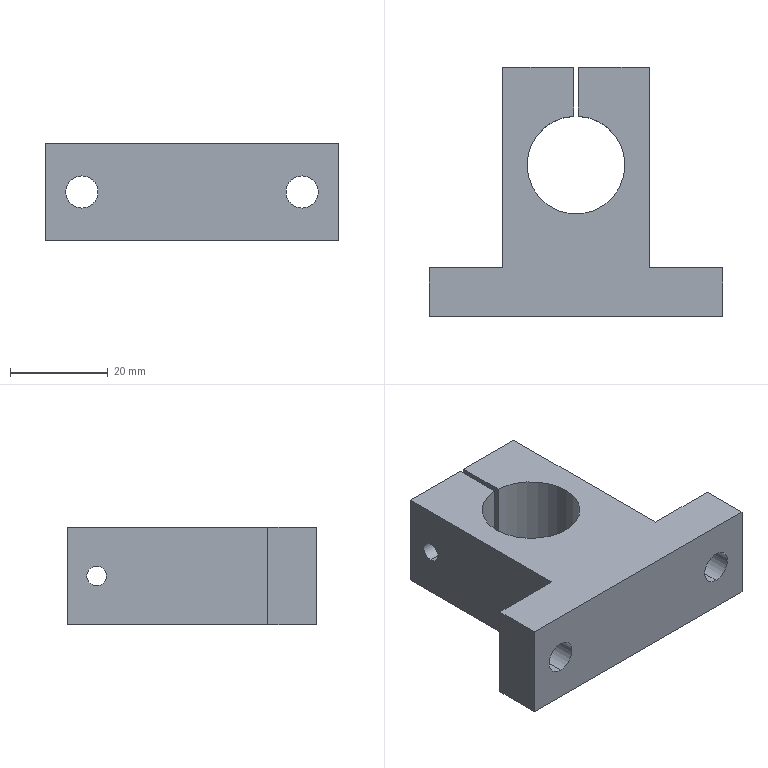Part | SolidWorks | features HoleWzd 3, Extrusion 1, RefAxis 1 | 1 solid | 27 faces | box 60 x 51 x 20 mm | volume 28604 mm3 | plane 14 | cylinder 13 | commonest cylinder face diameters 6.6 x4 20 x3 4 x2 5.5 x2 10 x2
STEP:
#1=CARTESIAN_POINT('',(-15.,45.,2.));
#2=VERTEX_POINT('',#1);
#3=CARTESIAN_POINT('',(-15.,45.,-2.));
#4=VERTEX_POINT('',#3);
#5=CARTESIAN_POINT('',(-15.,45.,0.));
#6=DIRECTION('',(1.,0.,0.));
#7=DIRECTION('',(0.,1.,0.));
#8=AXIS2_PLACEMENT_3D('',#5,#6,#7);
#9=CIRCLE('',#8,2.);
#10=EDGE_CURVE('',#2,#4,#9,.T.);
#11=ORIENTED_EDGE('',*,*,#10,.F.);
#12=CARTESIAN_POINT('',(-0.5,45.,2.));
#13=VERTEX_POINT('',#12);
#14=CARTESIAN_POINT('',(-0.5,45.,2.));
#15=DIRECTION('',(1.,0.,0.));
#16=VECTOR('',#15,1000.);
#17=LINE('',#14,#16);
#18=EDGE_CURVE('',#2,#13,#17,.T.);
#19=ORIENTED_EDGE('',*,*,#18,.T.);
#20=CARTESIAN_POINT('',(-0.5,45.,-2.));
#21=VERTEX_POINT('',#20);
#22=CARTESIAN_POINT('',(-0.5,45.,0.));
#23=DIRECTION('',(1.,0.,0.));
#24=DIRECTION('',(0.,0.,-1.));
#25=AXIS2_PLACEMENT_3D('',#22,#23,#24);
#26=CIRCLE('',#25,2.);
#27=EDGE_CURVE('',#13,#21,#26,.T.);
#28=ORIENTED_EDGE('',*,*,#27,.T.);
#29=CARTESIAN_POINT('',(-0.5,45.,-2.));
#30=DIRECTION('',(1.,0.,0.));
#31=VECTOR('',#30,1000.);
#32=LINE('',#29,#31);
#33=EDGE_CURVE('',#4,#21,#32,.T.);
#34=ORIENTED_EDGE('',*,*,#33,.F.);
#35=EDGE_LOOP('',(#11,#19,#28,#34));
#36=FACE_OUTER_BOUND('',#35,.T.);
#37=CARTESIAN_POINT('',(-0.5,45.,0.));
#38=DIRECTION('',(1.,0.,0.));
#39=DIRECTION('',(0.,0.,-1.));
#40=AXIS2_PLACEMENT_3D('',#37,#38,#39);
#41=CYLINDRICAL_SURFACE('',#40,2.);
#42=ADVANCED_FACE('',(#36),#41,.F.);
#43=CARTESIAN_POINT('',(-22.5,0.,-3.3));
#44=VERTEX_POINT('',#43);
#45=CARTESIAN_POINT('',(-22.5,0.,3.3));
#46=VERTEX_POINT('',#45);
#47=CARTESIAN_POINT('',(-22.5,0.,0.));
#48=DIRECTION('',(0.,1.,0.));
#49=DIRECTION('',(0.,0.,1.));
#50=AXIS2_PLACEMENT_3D('',#47,#48,#49);
#51=CIRCLE('',#50,3.3);
#52=EDGE_CURVE('',#44,#46,#51,.T.);
#53=ORIENTED_EDGE('',*,*,#52,.F.);
#54=CARTESIAN_POINT('',(-22.5,10.,-3.3));
#55=VERTEX_POINT('',#54);
#56=CARTESIAN_POINT('',(-22.5,10.,-3.3));
#57=DIRECTION('',(0.,1.,0.));
#58=VECTOR('',#57,1000.);
#59=LINE('',#56,#58);
#60=EDGE_CURVE('',#44,#55,#59,.T.);
#61=ORIENTED_EDGE('',*,*,#60,.T.);
#62=CARTESIAN_POINT('',(-22.5,10.,3.3));
#63=VERTEX_POINT('',#62);
#64=CARTESIAN_POINT('',(-22.5,10.,0.));
#65=DIRECTION('',(0.,1.,0.));
#66=DIRECTION('',(0.,0.,1.));
#67=AXIS2_PLACEMENT_3D('',#64,#65,#66);
#68=CIRCLE('',#67,3.3);
#69=EDGE_CURVE('',#55,#63,#68,.T.);
#70=ORIENTED_EDGE('',*,*,#69,.T.);
#71=CARTESIAN_POINT('',(-22.5,10.,3.3));
#72=DIRECTION('',(0.,1.,0.));
#73=VECTOR('',#72,1000.);
#74=LINE('',#71,#73);
#75=EDGE_CURVE('',#46,#63,#74,.T.);
#76=ORIENTED_EDGE('',*,*,#75,.F.);
#77=EDGE_LOOP('',(#53,#61,#70,#76));
#78=FACE_OUTER_BOUND('',#77,.T.);
#79=CARTESIAN_POINT('',(-22.5,10.,0.));
#80=DIRECTION('',(0.,1.,0.));
#81=DIRECTION('',(0.,0.,1.));
#82=AXIS2_PLACEMENT_3D('',#79,#80,#81);
#83=CYLINDRICAL_SURFACE('',#82,3.3);
#84=ADVANCED_FACE('',(#78),#83,.F.);
#85=CARTESIAN_POINT('',(22.5,0.,-3.3));
#86=VERTEX_POINT('',#85);
#87=CARTESIAN_POINT('',(22.5,0.,3.3));
#88=VERTEX_POINT('',#87);
#89=CARTESIAN_POINT('',(22.5,0.,0.));
#90=DIRECTION('',(0.,1.,0.));
#91=DIRECTION('',(0.,0.,1.));
#92=AXIS2_PLACEMENT_3D('',#89,#90,#91);
#93=CIRCLE('',#92,3.3);
#94=EDGE_CURVE('',#86,#88,#93,.T.);
#95=ORIENTED_EDGE('',*,*,#94,.F.);
#96=CARTESIAN_POINT('',(22.5,10.,-3.3));
#97=VERTEX_POINT('',#96);
#98=CARTESIAN_POINT('',(22.5,10.,-3.3));
#99=DIRECTION('',(0.,1.,0.));
#100=VECTOR('',#99,1000.);
#101=LINE('',#98,#100);
#102=EDGE_CURVE('',#86,#97,#101,.T.);
#103=ORIENTED_EDGE('',*,*,#102,.T.);
#104=CARTESIAN_POINT('',(22.5,10.,3.3));
#105=VERTEX_POINT('',#104);
#106=CARTESIAN_POINT('',(22.5,10.,0.));
#107=DIRECTION('',(0.,1.,0.));
#108=DIRECTION('',(0.,0.,1.));
#109=AXIS2_PLACEMENT_3D('',#106,#107,#108);
#110=CIRCLE('',#109,3.3);
#111=EDGE_CURVE('',#97,#105,#110,.T.);
#112=ORIENTED_EDGE('',*,*,#111,.T.);
#113=CARTESIAN_POINT('',(22.5,10.,3.3));
#114=DIRECTION('',(0.,1.,0.));
#115=VECTOR('',#114,1000.);
#116=LINE('',#113,#115);
#117=EDGE_CURVE('',#88,#105,#116,.T.);
#118=ORIENTED_EDGE('',*,*,#117,.F.);
#119=EDGE_LOOP('',(#95,#103,#112,#118));
#120=FACE_OUTER_BOUND('',#119,.T.);
#121=CARTESIAN_POINT('',(22.5,10.,0.));
#122=DIRECTION('',(0.,1.,0.));
#123=DIRECTION('',(0.,0.,1.));
#124=AXIS2_PLACEMENT_3D('',#121,#122,#123);
#125=CYLINDRICAL_SURFACE('',#124,3.3);
#126=ADVANCED_FACE('',(#120),#125,.F.);
#127=CARTESIAN_POINT('',(9.5,45.,5.));
#128=VERTEX_POINT('',#127);
#129=CARTESIAN_POINT('',(9.5,45.,-5.));
#130=VERTEX_POINT('',#129);
#131=CARTESIAN_POINT('',(9.5,45.,0.));
#132=DIRECTION('',(1.,0.,0.));
#133=DIRECTION('',(0.,0.,-1.));
#134=AXIS2_PLACEMENT_3D('',#131,#132,#133);
#135=CIRCLE('',#134,5.);
#136=EDGE_CURVE('',#128,#130,#135,.T.);
#137=ORIENTED_EDGE('',*,*,#136,.F.);
#138=CARTESIAN_POINT('',(15.,45.,5.));
#139=VERTEX_POINT('',#138);
#140=CARTESIAN_POINT('',(15.,45.,5.));
#141=DIRECTION('',(1.,0.,0.));
#142=VECTOR('',#141,1000.);
#143=LINE('',#140,#142);
#144=EDGE_CURVE('',#128,#139,#143,.T.);
#145=ORIENTED_EDGE('',*,*,#144,.T.);
#146=CARTESIAN_POINT('',(15.,45.,-5.));
#147=VERTEX_POINT('',#146);
#148=CARTESIAN_POINT('',(15.,45.,0.));
#149=DIRECTION('',(1.,0.,0.));
#150=DIRECTION('',(0.,0.,-1.));
#151=AXIS2_PLACEMENT_3D('',#148,#149,#150);
#152=CIRCLE('',#151,5.);
#153=EDGE_CURVE('',#139,#147,#152,.T.);
#154=ORIENTED_EDGE('',*,*,#153,.T.);
#155=CARTESIAN_POINT('',(15.,45.,-5.));
#156=DIRECTION('',(1.,0.,0.));
#157=VECTOR('',#156,1000.);
#158=LINE('',#155,#157);
#159=EDGE_CURVE('',#130,#147,#158,.T.);
#160=ORIENTED_EDGE('',*,*,#159,.F.);
#161=EDGE_LOOP('',(#137,#145,#154,#160));
#162=FACE_OUTER_BOUND('',#161,.T.);
#163=CARTESIAN_POINT('',(15.,45.,0.));
#164=DIRECTION('',(1.,0.,0.));
#165=DIRECTION('',(0.,0.,-1.));
#166=AXIS2_PLACEMENT_3D('',#163,#164,#165);
#167=CYLINDRICAL_SURFACE('',#166,5.);
#168=ADVANCED_FACE('',(#162),#167,.F.);
#169=CARTESIAN_POINT('',(0.5,45.,2.75));
#170=VERTEX_POINT('',#169);
#171=CARTESIAN_POINT('',(0.5,45.,-2.75));
#172=VERTEX_POINT('',#171);
#173=CARTESIAN_POINT('',(0.5,45.,0.));
#174=DIRECTION('',(1.,0.,0.));
#175=DIRECTION('',(0.,1.,0.));
#176=AXIS2_PLACEMENT_3D('',#173,#174,#175);
#177=CIRCLE('',#176,2.75);
#178=EDGE_CURVE('',#170,#172,#177,.T.);
#179=ORIENTED_EDGE('',*,*,#178,.F.);
#180=CARTESIAN_POINT('',(9.5,45.,2.75));
#181=VERTEX_POINT('',#180);
#182=CARTESIAN_POINT('',(15.,45.,2.75));
#183=DIRECTION('',(1.,0.,0.));
#184=VECTOR('',#183,1000.);
#185=LINE('',#182,#184);
#186=EDGE_CURVE('',#170,#181,#185,.T.);
#187=ORIENTED_EDGE('',*,*,#186,.T.);
#188=CARTESIAN_POINT('',(9.5,45.,-2.75));
#189=VERTEX_POINT('',#188);
#190=CARTESIAN_POINT('',(9.5,45.,0.));
#191=DIRECTION('',(1.,0.,0.));
#192=DIRECTION('',(0.,0.,-1.));
#193=AXIS2_PLACEMENT_3D('',#190,#191,#192);
#194=CIRCLE('',#193,2.75);
#195=EDGE_CURVE('',#181,#189,#194,.T.);
#196=ORIENTED_EDGE('',*,*,#195,.T.);
#197=CARTESIAN_POINT('',(15.,45.,-2.75));
#198=DIRECTION('',(1.,0.,0.));
#199=VECTOR('',#198,1000.);
#200=LINE('',#197,#199);
#201=EDGE_CURVE('',#172,#189,#200,.T.);
#202=ORIENTED_EDGE('',*,*,#201,.F.);
#203=EDGE_LOOP('',(#179,#187,#196,#202));
#204=FACE_OUTER_BOUND('',#203,.T.);
#205=CARTESIAN_POINT('',(15.,45.,0.));
#206=DIRECTION('',(1.,0.,0.));
#207=DIRECTION('',(0.,0.,-1.));
#208=AXIS2_PLACEMENT_3D('',#205,#206,#207);
#209=CYLINDRICAL_SURFACE('',#208,2.75);
#210=ADVANCED_FACE('',(#204),#209,.F.);
#211=CARTESIAN_POINT('',(10.,31.,10.));
#212=VERTEX_POINT('',#211);
#213=CARTESIAN_POINT('',(-10.,31.,10.));
#214=VERTEX_POINT('',#213);
#215=CARTESIAN_POINT('',(0.,31.,10.));
#216=DIRECTION('',(0.,0.,-1.));
#217=DIRECTION('',(1.,0.,0.));
#218=AXIS2_PLACEMENT_3D('',#215,#216,#217);
#219=CIRCLE('',#218,10.);
#220=EDGE_CURVE('',#212,#214,#219,.T.);
#221=ORIENTED_EDGE('',*,*,#220,.F.);
#222=CARTESIAN_POINT('',(10.,31.,-10.));
#223=VERTEX_POINT('',#222);
#224=CARTESIAN_POINT('',(10.,31.,10.));
#225=DIRECTION('',(0.,0.,-1.));
#226=VECTOR('',#225,1000.);
#227=LINE('',#224,#226);
#228=EDGE_CURVE('',#212,#223,#227,.T.);
#229=ORIENTED_EDGE('',*,*,#228,.T.);
#230=CARTESIAN_POINT('',(-10.,31.,-10.));
#231=VERTEX_POINT('',#230);
#232=CARTESIAN_POINT('',(0.,31.,-10.));
#233=DIRECTION('',(0.,0.,-1.));
#234=DIRECTION('',(1.,0.,0.));
#235=AXIS2_PLACEMENT_3D('',#232,#233,#234);
#236=CIRCLE('',#235,10.);
#237=EDGE_CURVE('',#223,#231,#236,.T.);
#238=ORIENTED_EDGE('',*,*,#237,.T.);
#239=CARTESIAN_POINT('',(-10.,31.,10.));
#240=DIRECTION('',(0.,0.,-1.));
#241=VECTOR('',#240,1000.);
#242=LINE('',#239,#241);
#243=EDGE_CURVE('',#214,#231,#242,.T.);
#244=ORIENTED_EDGE('',*,*,#243,.F.);
#245=EDGE_LOOP('',(#221,#229,#238,#244));
#246=FACE_OUTER_BOUND('',#245,.T.);
#247=CARTESIAN_POINT('',(0.,31.,10.));
#248=DIRECTION('',(0.,0.,-1.));
#249=DIRECTION('',(-1.,0.,0.));
#250=AXIS2_PLACEMENT_3D('',#247,#248,#249);
#251=CYLINDRICAL_SURFACE('',#250,10.);
#252=ADVANCED_FACE('',(#246),#251,.F.);
#253=CARTESIAN_POINT('',(-0.5,40.987,10.));
#254=VERTEX_POINT('',#253);
#255=CARTESIAN_POINT('',(0.,31.,10.));
#256=DIRECTION('',(0.,0.,-1.));
#257=DIRECTION('',(1.,0.,0.));
#258=AXIS2_PLACEMENT_3D('',#255,#256,#257);
#259=CIRCLE('',#258,10.);
#260=EDGE_CURVE('',#214,#254,#259,.T.);
#261=ORIENTED_EDGE('',*,*,#260,.F.);
#262=ORIENTED_EDGE('',*,*,#243,.T.);
#263=CARTESIAN_POINT('',(-0.5,40.987,-10.));
#264=VERTEX_POINT('',#263);
#265=CARTESIAN_POINT('',(0.,31.,-10.));
#266=DIRECTION('',(0.,0.,-1.));
#267=DIRECTION('',(1.,0.,0.));
#268=AXIS2_PLACEMENT_3D('',#265,#266,#267);
#269=CIRCLE('',#268,10.);
#270=EDGE_CURVE('',#231,#264,#269,.T.);
#271=ORIENTED_EDGE('',*,*,#270,.T.);
#272=CARTESIAN_POINT('',(-0.5,40.987,10.));
#273=DIRECTION('',(0.,0.,-1.));
#274=VECTOR('',#273,1000.);
#275=LINE('',#272,#274);
#276=EDGE_CURVE('',#254,#264,#275,.T.);
#277=ORIENTED_EDGE('',*,*,#276,.F.);
#278=EDGE_LOOP('',(#261,#262,#271,#277));
#279=FACE_OUTER_BOUND('',#278,.T.);
#280=CARTESIAN_POINT('',(0.,31.,10.));
#281=DIRECTION('',(0.,0.,-1.));
#282=DIRECTION('',(-1.,0.,0.));
#283=AXIS2_PLACEMENT_3D('',#280,#281,#282);
#284=CYLINDRICAL_SURFACE('',#283,10.);
#285=ADVANCED_FACE('',(#279),#284,.F.);
#286=CARTESIAN_POINT('',(15.,10.,-10.));
#287=VERTEX_POINT('',#286);
#288=CARTESIAN_POINT('',(15.,51.,-10.));
#289=VERTEX_POINT('',#288);
#290=CARTESIAN_POINT('',(15.,10.,-10.));
#291=DIRECTION('',(0.,1.,0.));
#292=VECTOR('',#291,1000.);
#293=LINE('',#290,#292);
#294=EDGE_CURVE('',#287,#289,#293,.T.);
#295=ORIENTED_EDGE('',*,*,#294,.T.);
#296=CARTESIAN_POINT('',(15.,51.,10.));
#297=VERTEX_POINT('',#296);
#298=CARTESIAN_POINT('',(15.,51.,10.));
#299=DIRECTION('',(0.,0.,-1.));
#300=VECTOR('',#299,1000.);
#301=LINE('',#298,#300);
#302=EDGE_CURVE('',#297,#289,#301,.T.);
#303=ORIENTED_EDGE('',*,*,#302,.F.);
#304=CARTESIAN_POINT('',(15.,10.,10.));
#305=VERTEX_POINT('',#304);
#306=CARTESIAN_POINT('',(15.,10.,10.));
#307=DIRECTION('',(0.,1.,0.));
#308=VECTOR('',#307,1000.);
#309=LINE('',#306,#308);
#310=EDGE_CURVE('',#305,#297,#309,.T.);
#311=ORIENTED_EDGE('',*,*,#310,.F.);
#312=CARTESIAN_POINT('',(15.,10.,10.));
#313=DIRECTION('',(0.,0.,-1.));
#314=VECTOR('',#313,1000.);
#315=LINE('',#312,#314);
#316=EDGE_CURVE('',#305,#287,#315,.T.);
#317=ORIENTED_EDGE('',*,*,#316,.T.);
#318=EDGE_LOOP('',(#295,#303,#311,#317));
#319=FACE_OUTER_BOUND('',#318,.T.);
#320=CARTESIAN_POINT('',(15.,45.,0.));
#321=DIRECTION('',(1.,0.,0.));
#322=DIRECTION('',(0.,0.,-1.));
#323=AXIS2_PLACEMENT_3D('',#320,#321,#322);
#324=CIRCLE('',#323,5.);
#325=EDGE_CURVE('',#147,#139,#324,.T.);
#326=ORIENTED_EDGE('',*,*,#325,.F.);
#327=ORIENTED_EDGE('',*,*,#153,.F.);
#328=EDGE_LOOP('',(#326,#327));
#329=FACE_BOUND('',#328,.T.);
#330=CARTESIAN_POINT('',(15.,10.,10.));
#331=DIRECTION('',(-1.,0.,0.));
#332=DIRECTION('',(0.,-1.,0.));
#333=AXIS2_PLACEMENT_3D('',#330,#331,#332);
#334=PLANE('',#333);
#335=ADVANCED_FACE('',(#319,#329),#334,.F.);
#336=CARTESIAN_POINT('',(-30.,10.,-10.));
#337=VERTEX_POINT('',#336);
#338=CARTESIAN_POINT('',(-30.,0.,-10.));
#339=VERTEX_POINT('',#338);
#340=CARTESIAN_POINT('',(-30.,0.,-10.));
#341=DIRECTION('',(0.,-1.,0.));
#342=VECTOR('',#341,1000.);
#343=LINE('',#340,#342);
#344=EDGE_CURVE('',#337,#339,#343,.T.);
#345=ORIENTED_EDGE('',*,*,#344,.T.);
#346=CARTESIAN_POINT('',(-30.,0.,10.));
#347=VERTEX_POINT('',#346);
#348=CARTESIAN_POINT('',(-30.,0.,10.));
#349=DIRECTION('',(0.,0.,-1.));
#350=VECTOR('',#349,1000.);
#351=LINE('',#348,#350);
#352=EDGE_CURVE('',#347,#339,#351,.T.);
#353=ORIENTED_EDGE('',*,*,#352,.F.);
#354=CARTESIAN_POINT('',(-30.,10.,10.));
#355=VERTEX_POINT('',#354);
#356=CARTESIAN_POINT('',(-30.,0.,10.));
#357=DIRECTION('',(0.,-1.,0.));
#358=VECTOR('',#357,1000.);
#359=LINE('',#356,#358);
#360=EDGE_CURVE('',#355,#347,#359,.T.);
#361=ORIENTED_EDGE('',*,*,#360,.F.);
#362=CARTESIAN_POINT('',(-30.,10.,10.));
#363=DIRECTION('',(0.,0.,-1.));
#364=VECTOR('',#363,1000.);
#365=LINE('',#362,#364);
#366=EDGE_CURVE('',#355,#337,#365,.T.);
#367=ORIENTED_EDGE('',*,*,#366,.T.);
#368=EDGE_LOOP('',(#345,#353,#361,#367));
#369=FACE_OUTER_BOUND('',#368,.T.);
#370=CARTESIAN_POINT('',(-30.,0.,10.));
#371=DIRECTION('',(1.,0.,0.));
#372=DIRECTION('',(0.,0.,-1.));
#373=AXIS2_PLACEMENT_3D('',#370,#371,#372);
#374=PLANE('',#373);
#375=ADVANCED_FACE('',(#369),#374,.F.);
#376=CARTESIAN_POINT('',(-22.5,0.,0.));
#377=DIRECTION('',(0.,1.,0.));
#378=DIRECTION('',(0.,0.,1.));
#379=AXIS2_PLACEMENT_3D('',#376,#377,#378);
#380=CIRCLE('',#379,3.3);
#381=EDGE_CURVE('',#46,#44,#380,.T.);
#382=ORIENTED_EDGE('',*,*,#381,.T.);
#383=ORIENTED_EDGE('',*,*,#52,.T.);
#384=EDGE_LOOP('',(#382,#383));
#385=FACE_BOUND('',#384,.T.);
#386=CARTESIAN_POINT('',(22.5,0.,0.));
#387=DIRECTION('',(0.,1.,0.));
#388=DIRECTION('',(0.,0.,1.));
#389=AXIS2_PLACEMENT_3D('',#386,#387,#388);
#390=CIRCLE('',#389,3.3);
#391=EDGE_CURVE('',#88,#86,#390,.T.);
#392=ORIENTED_EDGE('',*,*,#391,.T.);
#393=ORIENTED_EDGE('',*,*,#94,.T.);
#394=EDGE_LOOP('',(#392,#393));
#395=FACE_BOUND('',#394,.T.);
#396=CARTESIAN_POINT('',(30.,0.,-10.));
#397=VERTEX_POINT('',#396);
#398=CARTESIAN_POINT('',(30.,0.,-10.));
#399=DIRECTION('',(1.,0.,0.));
#400=VECTOR('',#399,1000.);
#401=LINE('',#398,#400);
#402=EDGE_CURVE('',#339,#397,#401,.T.);
#403=ORIENTED_EDGE('',*,*,#402,.T.);
#404=CARTESIAN_POINT('',(30.,0.,10.));
#405=VERTEX_POINT('',#404);
#406=CARTESIAN_POINT('',(30.,0.,10.));
#407=DIRECTION('',(0.,0.,-1.));
#408=VECTOR('',#407,1000.);
#409=LINE('',#406,#408);
#410=EDGE_CURVE('',#405,#397,#409,.T.);
#411=ORIENTED_EDGE('',*,*,#410,.F.);
#412=CARTESIAN_POINT('',(30.,0.,10.));
#413=DIRECTION('',(1.,0.,0.));
#414=VECTOR('',#413,1000.);
#415=LINE('',#412,#414);
#416=EDGE_CURVE('',#347,#405,#415,.T.);
#417=ORIENTED_EDGE('',*,*,#416,.F.);
#418=ORIENTED_EDGE('',*,*,#352,.T.);
#419=EDGE_LOOP('',(#403,#411,#417,#418));
#420=FACE_OUTER_BOUND('',#419,.T.);
#421=CARTESIAN_POINT('',(30.,0.,10.));
#422=DIRECTION('',(0.,1.,0.));
#423=DIRECTION('',(-1.,0.,0.));
#424=AXIS2_PLACEMENT_3D('',#421,#422,#423);
#425=PLANE('',#424);
#426=ADVANCED_FACE('',(#385,#395,#420),#425,.F.);
#427=CARTESIAN_POINT('',(30.,10.,-10.));
#428=VERTEX_POINT('',#427);
#429=CARTESIAN_POINT('',(30.,0.,-10.));
#430=DIRECTION('',(0.,1.,0.));
#431=VECTOR('',#430,1000.);
#432=LINE('',#429,#431);
#433=EDGE_CURVE('',#397,#428,#432,.T.);
#434=ORIENTED_EDGE('',*,*,#433,.T.);
#435=CARTESIAN_POINT('',(30.,10.,10.));
#436=VERTEX_POINT('',#435);
#437=CARTESIAN_POINT('',(30.,10.,10.));
#438=DIRECTION('',(0.,0.,-1.));
#439=VECTOR('',#438,1000.);
#440=LINE('',#437,#439);
#441=EDGE_CURVE('',#436,#428,#440,.T.);
#442=ORIENTED_EDGE('',*,*,#441,.F.);
#443=CARTESIAN_POINT('',(30.,0.,10.));
#444=DIRECTION('',(0.,1.,0.));
#445=VECTOR('',#444,1000.);
#446=LINE('',#443,#445);
#447=EDGE_CURVE('',#405,#436,#446,.T.);
#448=ORIENTED_EDGE('',*,*,#447,.F.);
#449=ORIENTED_EDGE('',*,*,#410,.T.);
#450=EDGE_LOOP('',(#434,#442,#448,#449));
#451=FACE_OUTER_BOUND('',#450,.T.);
#452=CARTESIAN_POINT('',(30.,0.,10.));
#453=DIRECTION('',(-1.,0.,0.));
#454=DIRECTION('',(0.,0.,1.));
#455=AXIS2_PLACEMENT_3D('',#452,#453,#454);
#456=PLANE('',#455);
#457=ADVANCED_FACE('',(#451),#456,.F.);
#458=CARTESIAN_POINT('',(22.5,10.,0.));
#459=DIRECTION('',(0.,1.,0.));
#460=DIRECTION('',(0.,0.,1.));
#461=AXIS2_PLACEMENT_3D('',#458,#459,#460);
#462=CIRCLE('',#461,3.3);
#463=EDGE_CURVE('',#105,#97,#462,.T.);
#464=ORIENTED_EDGE('',*,*,#463,.F.);
#465=ORIENTED_EDGE('',*,*,#111,.F.);
#466=EDGE_LOOP('',(#464,#465));
#467=FACE_BOUND('',#466,.T.);
#468=CARTESIAN_POINT('',(30.,10.,-10.));
#469=DIRECTION('',(-1.,0.,0.));
#470=VECTOR('',#469,1000.);
#471=LINE('',#468,#470);
#472=EDGE_CURVE('',#428,#287,#471,.T.);
#473=ORIENTED_EDGE('',*,*,#472,.T.);
#474=ORIENTED_EDGE('',*,*,#316,.F.);
#475=CARTESIAN_POINT('',(30.,10.,10.));
#476=DIRECTION('',(-1.,0.,0.));
#477=VECTOR('',#476,1000.);
#478=LINE('',#475,#477);
#479=EDGE_CURVE('',#436,#305,#478,.T.);
#480=ORIENTED_EDGE('',*,*,#479,.F.);
#481=ORIENTED_EDGE('',*,*,#441,.T.);
#482=EDGE_LOOP('',(#473,#474,#480,#481));
#483=FACE_OUTER_BOUND('',#482,.T.);
#484=CARTESIAN_POINT('',(30.,10.,10.));
#485=DIRECTION('',(0.,-1.,0.));
#486=DIRECTION('',(1.,0.,0.));
#487=AXIS2_PLACEMENT_3D('',#484,#485,#486);
#488=PLANE('',#487);
#489=ADVANCED_FACE('',(#467,#483),#488,.F.);
#490=CARTESIAN_POINT('',(0.5,51.,-10.));
#491=VERTEX_POINT('',#490);
#492=CARTESIAN_POINT('',(0.5,51.,-10.));
#493=DIRECTION('',(-1.,0.,0.));
#494=VECTOR('',#493,1000.);
#495=LINE('',#492,#494);
#496=EDGE_CURVE('',#289,#491,#495,.T.);
#497=ORIENTED_EDGE('',*,*,#496,.T.);
#498=CARTESIAN_POINT('',(0.5,51.,10.));
#499=VERTEX_POINT('',#498);
#500=CARTESIAN_POINT('',(0.5,51.,10.));
#501=DIRECTION('',(0.,0.,-1.));
#502=VECTOR('',#501,1000.);
#503=LINE('',#500,#502);
#504=EDGE_CURVE('',#499,#491,#503,.T.);
#505=ORIENTED_EDGE('',*,*,#504,.F.);
#506=CARTESIAN_POINT('',(0.5,51.,10.));
#507=DIRECTION('',(-1.,0.,0.));
#508=VECTOR('',#507,1000.);
#509=LINE('',#506,#508);
#510=EDGE_CURVE('',#297,#499,#509,.T.);
#511=ORIENTED_EDGE('',*,*,#510,.F.);
#512=ORIENTED_EDGE('',*,*,#302,.T.);
#513=EDGE_LOOP('',(#497,#505,#511,#512));
#514=FACE_OUTER_BOUND('',#513,.T.);
#515=CARTESIAN_POINT('',(0.5,51.,10.));
#516=DIRECTION('',(0.,-1.,0.));
#517=DIRECTION('',(1.,0.,0.));
#518=AXIS2_PLACEMENT_3D('',#515,#516,#517);
#519=PLANE('',#518);
#520=ADVANCED_FACE('',(#514),#519,.F.);
#521=CARTESIAN_POINT('',(0.5,45.,0.));
#522=DIRECTION('',(1.,0.,0.));
#523=DIRECTION('',(0.,1.,0.));
#524=AXIS2_PLACEMENT_3D('',#521,#522,#523);
#525=CIRCLE('',#524,2.75);
#526=EDGE_CURVE('',#172,#170,#525,.T.);
#527=ORIENTED_EDGE('',*,*,#526,.T.);
#528=ORIENTED_EDGE('',*,*,#178,.T.);
#529=EDGE_LOOP('',(#527,#528));
#530=FACE_BOUND('',#529,.T.);
#531=CARTESIAN_POINT('',(0.5,40.987,-10.));
#532=VERTEX_POINT('',#531);
#533=CARTESIAN_POINT('',(0.5,40.987,-10.));
#534=DIRECTION('',(0.,-1.,0.));
#535=VECTOR('',#534,1000.);
#536=LINE('',#533,#535);
#537=EDGE_CURVE('',#491,#532,#536,.T.);
#538=ORIENTED_EDGE('',*,*,#537,.T.);
#539=CARTESIAN_POINT('',(0.5,40.987,10.));
#540=VERTEX_POINT('',#539);
#541=CARTESIAN_POINT('',(0.5,40.987,10.));
#542=DIRECTION('',(0.,0.,-1.));
#543=VECTOR('',#542,1000.);
#544=LINE('',#541,#543);
#545=EDGE_CURVE('',#540,#532,#544,.T.);
#546=ORIENTED_EDGE('',*,*,#545,.F.);
#547=CARTESIAN_POINT('',(0.5,40.987,10.));
#548=DIRECTION('',(0.,-1.,0.));
#549=VECTOR('',#548,1000.);
#550=LINE('',#547,#549);
#551=EDGE_CURVE('',#499,#540,#550,.T.);
#552=ORIENTED_EDGE('',*,*,#551,.F.);
#553=ORIENTED_EDGE('',*,*,#504,.T.);
#554=EDGE_LOOP('',(#538,#546,#552,#553));
#555=FACE_OUTER_BOUND('',#554,.T.);
#556=CARTESIAN_POINT('',(0.5,40.987,10.));
#557=DIRECTION('',(1.,0.,0.));
#558=DIRECTION('',(0.,1.,0.));
#559=AXIS2_PLACEMENT_3D('',#556,#557,#558);
#560=PLANE('',#559);
#561=ADVANCED_FACE('',(#530,#555),#560,.F.);
#562=ORIENTED_EDGE('',*,*,#228,.F.);
#563=CARTESIAN_POINT('',(0.,31.,10.));
#564=DIRECTION('',(0.,0.,-1.));
#565=DIRECTION('',(1.,0.,0.));
#566=AXIS2_PLACEMENT_3D('',#563,#564,#565);
#567=CIRCLE('',#566,10.);
#568=EDGE_CURVE('',#540,#212,#567,.T.);
#569=ORIENTED_EDGE('',*,*,#568,.F.);
#570=ORIENTED_EDGE('',*,*,#545,.T.);
#571=CARTESIAN_POINT('',(0.,31.,-10.));
#572=DIRECTION('',(0.,0.,-1.));
#573=DIRECTION('',(1.,0.,0.));
#574=AXIS2_PLACEMENT_3D('',#571,#572,#573);
#575=CIRCLE('',#574,10.);
#576=EDGE_CURVE('',#532,#223,#575,.T.);
#577=ORIENTED_EDGE('',*,*,#576,.T.);
#578=EDGE_LOOP('',(#562,#569,#570,#577));
#579=FACE_OUTER_BOUND('',#578,.T.);
#580=CARTESIAN_POINT('',(0.,31.,10.));
#581=DIRECTION('',(0.,0.,-1.));
#582=DIRECTION('',(-1.,0.,0.));
#583=AXIS2_PLACEMENT_3D('',#580,#581,#582);
#584=CYLINDRICAL_SURFACE('',#583,10.);
#585=ADVANCED_FACE('',(#579),#584,.F.);
#586=CARTESIAN_POINT('',(-0.5,45.,0.));
#587=DIRECTION('',(1.,0.,0.));
#588=DIRECTION('',(0.,0.,-1.));
#589=AXIS2_PLACEMENT_3D('',#586,#587,#588);
#590=CIRCLE('',#589,2.);
#591=EDGE_CURVE('',#21,#13,#590,.T.);
#592=ORIENTED_EDGE('',*,*,#591,.F.);
#593=ORIENTED_EDGE('',*,*,#27,.F.);
#594=EDGE_LOOP('',(#592,#593));
#595=FACE_BOUND('',#594,.T.);
#596=CARTESIAN_POINT('',(-0.5,51.,-10.));
#597=VERTEX_POINT('',#596);
#598=CARTESIAN_POINT('',(-0.5,40.987,-10.));
#599=DIRECTION('',(0.,1.,0.));
#600=VECTOR('',#599,1000.);
#601=LINE('',#598,#600);
#602=EDGE_CURVE('',#264,#597,#601,.T.);
#603=ORIENTED_EDGE('',*,*,#602,.T.);
#604=CARTESIAN_POINT('',(-0.5,51.,10.));
#605=VERTEX_POINT('',#604);
#606=CARTESIAN_POINT('',(-0.5,51.,10.));
#607=DIRECTION('',(0.,0.,-1.));
#608=VECTOR('',#607,1000.);
#609=LINE('',#606,#608);
#610=EDGE_CURVE('',#605,#597,#609,.T.);
#611=ORIENTED_EDGE('',*,*,#610,.F.);
#612=CARTESIAN_POINT('',(-0.5,40.987,10.));
#613=DIRECTION('',(0.,1.,0.));
#614=VECTOR('',#613,1000.);
#615=LINE('',#612,#614);
#616=EDGE_CURVE('',#254,#605,#615,.T.);
#617=ORIENTED_EDGE('',*,*,#616,.F.);
#618=ORIENTED_EDGE('',*,*,#276,.T.);
#619=EDGE_LOOP('',(#603,#611,#617,#618));
#620=FACE_OUTER_BOUND('',#619,.T.);
#621=CARTESIAN_POINT('',(-0.5,40.987,10.));
#622=DIRECTION('',(-1.,0.,0.));
#623=DIRECTION('',(0.,-1.,0.));
#624=AXIS2_PLACEMENT_3D('',#621,#622,#623);
#625=PLANE('',#624);
#626=ADVANCED_FACE('',(#595,#620),#625,.F.);
#627=CARTESIAN_POINT('',(-15.,51.,-10.));
#628=VERTEX_POINT('',#627);
#629=CARTESIAN_POINT('',(-15.,51.,-10.));
#630=DIRECTION('',(-1.,0.,0.));
#631=VECTOR('',#630,1000.);
#632=LINE('',#629,#631);
#633=EDGE_CURVE('',#597,#628,#632,.T.);
#634=ORIENTED_EDGE('',*,*,#633,.T.);
#635=CARTESIAN_POINT('',(-15.,51.,10.));
#636=VERTEX_POINT('',#635);
#637=CARTESIAN_POINT('',(-15.,51.,10.));
#638=DIRECTION('',(0.,0.,-1.));
#639=VECTOR('',#638,1000.);
#640=LINE('',#637,#639);
#641=EDGE_CURVE('',#636,#628,#640,.T.);
#642=ORIENTED_EDGE('',*,*,#641,.F.);
#643=CARTESIAN_POINT('',(-15.,51.,10.));
#644=DIRECTION('',(-1.,0.,0.));
#645=VECTOR('',#644,1000.);
#646=LINE('',#643,#645);
#647=EDGE_CURVE('',#605,#636,#646,.T.);
#648=ORIENTED_EDGE('',*,*,#647,.F.);
#649=ORIENTED_EDGE('',*,*,#610,.T.);
#650=EDGE_LOOP('',(#634,#642,#648,#649));
#651=FACE_OUTER_BOUND('',#650,.T.);
#652=CARTESIAN_POINT('',(-15.,51.,10.));
#653=DIRECTION('',(0.,-1.,0.));
#654=DIRECTION('',(0.,0.,-1.));
#655=AXIS2_PLACEMENT_3D('',#652,#653,#654);
#656=PLANE('',#655);
#657=ADVANCED_FACE('',(#651),#656,.F.);
#658=CARTESIAN_POINT('',(-15.,45.,0.));
#659=DIRECTION('',(1.,0.,0.));
#660=DIRECTION('',(0.,1.,0.));
#661=AXIS2_PLACEMENT_3D('',#658,#659,#660);
#662=CIRCLE('',#661,2.);
#663=EDGE_CURVE('',#4,#2,#662,.T.);
#664=ORIENTED_EDGE('',*,*,#663,.T.);
#665=ORIENTED_EDGE('',*,*,#10,.T.);
#666=EDGE_LOOP('',(#664,#665));
#667=FACE_BOUND('',#666,.T.);
#668=CARTESIAN_POINT('',(-15.,10.,-10.));
#669=VERTEX_POINT('',#668);
#670=CARTESIAN_POINT('',(-15.,10.,-10.));
#671=DIRECTION('',(0.,-1.,0.));
#672=VECTOR('',#671,1000.);
#673=LINE('',#670,#672);
#674=EDGE_CURVE('',#628,#669,#673,.T.);
#675=ORIENTED_EDGE('',*,*,#674,.T.);
#676=CARTESIAN_POINT('',(-15.,10.,10.));
#677=VERTEX_POINT('',#676);
#678=CARTESIAN_POINT('',(-15.,10.,10.));
#679=DIRECTION('',(0.,0.,-1.));
#680=VECTOR('',#679,1000.);
#681=LINE('',#678,#680);
#682=EDGE_CURVE('',#677,#669,#681,.T.);
#683=ORIENTED_EDGE('',*,*,#682,.F.);
#684=CARTESIAN_POINT('',(-15.,10.,10.));
#685=DIRECTION('',(0.,-1.,0.));
#686=VECTOR('',#685,1000.);
#687=LINE('',#684,#686);
#688=EDGE_CURVE('',#636,#677,#687,.T.);
#689=ORIENTED_EDGE('',*,*,#688,.F.);
#690=ORIENTED_EDGE('',*,*,#641,.T.);
#691=EDGE_LOOP('',(#675,#683,#689,#690));
#692=FACE_OUTER_BOUND('',#691,.T.);
#693=CARTESIAN_POINT('',(-15.,10.,10.));
#694=DIRECTION('',(1.,0.,0.));
#695=DIRECTION('',(0.,1.,0.));
#696=AXIS2_PLACEMENT_3D('',#693,#694,#695);
#697=PLANE('',#696);
#698=ADVANCED_FACE('',(#667,#692),#697,.F.);
#699=CARTESIAN_POINT('',(-22.5,10.,0.));
#700=DIRECTION('',(0.,1.,0.));
#701=DIRECTION('',(0.,0.,1.));
#702=AXIS2_PLACEMENT_3D('',#699,#700,#701);
#703=CIRCLE('',#702,3.3);
#704=EDGE_CURVE('',#63,#55,#703,.T.);
#705=ORIENTED_EDGE('',*,*,#704,.F.);
#706=ORIENTED_EDGE('',*,*,#69,.F.);
#707=EDGE_LOOP('',(#705,#706));
#708=FACE_BOUND('',#707,.T.);
#709=CARTESIAN_POINT('',(-30.,10.,-10.));
#710=DIRECTION('',(-1.,0.,0.));
#711=VECTOR('',#710,1000.);
#712=LINE('',#709,#711);
#713=EDGE_CURVE('',#669,#337,#712,.T.);
#714=ORIENTED_EDGE('',*,*,#713,.T.);
#715=ORIENTED_EDGE('',*,*,#366,.F.);
#716=CARTESIAN_POINT('',(-30.,10.,10.));
#717=DIRECTION('',(-1.,0.,0.));
#718=VECTOR('',#717,1000.);
#719=LINE('',#716,#718);
#720=EDGE_CURVE('',#677,#355,#719,.T.);
#721=ORIENTED_EDGE('',*,*,#720,.F.);
#722=ORIENTED_EDGE('',*,*,#682,.T.);
#723=EDGE_LOOP('',(#714,#715,#721,#722));
#724=FACE_OUTER_BOUND('',#723,.T.);
#725=CARTESIAN_POINT('',(-30.,10.,10.));
#726=DIRECTION('',(0.,-1.,0.));
#727=DIRECTION('',(0.,0.,-1.));
#728=AXIS2_PLACEMENT_3D('',#725,#726,#727);
#729=PLANE('',#728);
#730=ADVANCED_FACE('',(#708,#724),#729,.F.);
#731=ORIENTED_EDGE('',*,*,#360,.T.);
#732=ORIENTED_EDGE('',*,*,#416,.T.);
#733=ORIENTED_EDGE('',*,*,#447,.T.);
#734=ORIENTED_EDGE('',*,*,#479,.T.);
#735=ORIENTED_EDGE('',*,*,#310,.T.);
#736=ORIENTED_EDGE('',*,*,#510,.T.);
#737=ORIENTED_EDGE('',*,*,#551,.T.);
#738=ORIENTED_EDGE('',*,*,#568,.T.);
#739=ORIENTED_EDGE('',*,*,#220,.T.);
#740=ORIENTED_EDGE('',*,*,#260,.T.);
#741=ORIENTED_EDGE('',*,*,#616,.T.);
#742=ORIENTED_EDGE('',*,*,#647,.T.);
#743=ORIENTED_EDGE('',*,*,#688,.T.);
#744=ORIENTED_EDGE('',*,*,#720,.T.);
#745=EDGE_LOOP('',(#731,#732,#733,#734,#735,#736,#737,#738,#739,#740,#741,#742,#743,#744));
#746=FACE_OUTER_BOUND('',#745,.T.);
#747=CARTESIAN_POINT('',(0.,31.,10.));
#748=DIRECTION('',(0.,0.,1.));
#749=DIRECTION('',(1.,0.,0.));
#750=AXIS2_PLACEMENT_3D('',#747,#748,#749);
#751=PLANE('',#750);
#752=ADVANCED_FACE('',(#746),#751,.T.);
#753=ORIENTED_EDGE('',*,*,#344,.F.);
#754=ORIENTED_EDGE('',*,*,#713,.F.);
#755=ORIENTED_EDGE('',*,*,#674,.F.);
#756=ORIENTED_EDGE('',*,*,#633,.F.);
#757=ORIENTED_EDGE('',*,*,#602,.F.);
#758=ORIENTED_EDGE('',*,*,#270,.F.);
#759=ORIENTED_EDGE('',*,*,#237,.F.);
#760=ORIENTED_EDGE('',*,*,#576,.F.);
#761=ORIENTED_EDGE('',*,*,#537,.F.);
#762=ORIENTED_EDGE('',*,*,#496,.F.);
#763=ORIENTED_EDGE('',*,*,#294,.F.);
#764=ORIENTED_EDGE('',*,*,#472,.F.);
#765=ORIENTED_EDGE('',*,*,#433,.F.);
#766=ORIENTED_EDGE('',*,*,#402,.F.);
#767=EDGE_LOOP('',(#753,#754,#755,#756,#757,#758,#759,#760,#761,#762,#763,#764,#765,#766));
#768=FACE_OUTER_BOUND('',#767,.T.);
#769=CARTESIAN_POINT('',(0.,31.,-10.));
#770=DIRECTION('',(0.,0.,1.));
#771=DIRECTION('',(1.,0.,0.));
#772=AXIS2_PLACEMENT_3D('',#769,#770,#771);
#773=PLANE('',#772);
#774=ADVANCED_FACE('',(#768),#773,.F.);
#775=ORIENTED_EDGE('',*,*,#186,.F.);
#776=ORIENTED_EDGE('',*,*,#526,.F.);
#777=ORIENTED_EDGE('',*,*,#201,.T.);
#778=CARTESIAN_POINT('',(9.5,45.,0.));
#779=DIRECTION('',(1.,0.,0.));
#780=DIRECTION('',(0.,0.,-1.));
#781=AXIS2_PLACEMENT_3D('',#778,#779,#780);
#782=CIRCLE('',#781,2.75);
#783=EDGE_CURVE('',#189,#181,#782,.T.);
#784=ORIENTED_EDGE('',*,*,#783,.T.);
#785=EDGE_LOOP('',(#775,#776,#777,#784));
#786=FACE_OUTER_BOUND('',#785,.T.);
#787=CARTESIAN_POINT('',(15.,45.,0.));
#788=DIRECTION('',(1.,0.,0.));
#789=DIRECTION('',(0.,0.,-1.));
#790=AXIS2_PLACEMENT_3D('',#787,#788,#789);
#791=CYLINDRICAL_SURFACE('',#790,2.75);
#792=ADVANCED_FACE('',(#786),#791,.F.);
#793=ORIENTED_EDGE('',*,*,#783,.F.);
#794=ORIENTED_EDGE('',*,*,#195,.F.);
#795=EDGE_LOOP('',(#793,#794));
#796=FACE_BOUND('',#795,.T.);
#797=CARTESIAN_POINT('',(9.5,45.,0.));
#798=DIRECTION('',(1.,0.,0.));
#799=DIRECTION('',(0.,0.,-1.));
#800=AXIS2_PLACEMENT_3D('',#797,#798,#799);
#801=CIRCLE('',#800,5.);
#802=EDGE_CURVE('',#130,#128,#801,.T.);
#803=ORIENTED_EDGE('',*,*,#802,.T.);
#804=ORIENTED_EDGE('',*,*,#136,.T.);
#805=EDGE_LOOP('',(#803,#804));
#806=FACE_OUTER_BOUND('',#805,.T.);
#807=CARTESIAN_POINT('',(9.5,47.75,0.));
#808=DIRECTION('',(-1.,0.,0.));
#809=DIRECTION('',(0.,0.,1.));
#810=AXIS2_PLACEMENT_3D('',#807,#808,#809);
#811=PLANE('',#810);
#812=ADVANCED_FACE('',(#796,#806),#811,.F.);
#813=ORIENTED_EDGE('',*,*,#144,.F.);
#814=ORIENTED_EDGE('',*,*,#802,.F.);
#815=ORIENTED_EDGE('',*,*,#159,.T.);
#816=ORIENTED_EDGE('',*,*,#325,.T.);
#817=EDGE_LOOP('',(#813,#814,#815,#816));
#818=FACE_OUTER_BOUND('',#817,.T.);
#819=CARTESIAN_POINT('',(15.,45.,0.));
#820=DIRECTION('',(1.,0.,0.));
#821=DIRECTION('',(0.,0.,-1.));
#822=AXIS2_PLACEMENT_3D('',#819,#820,#821);
#823=CYLINDRICAL_SURFACE('',#822,5.);
#824=ADVANCED_FACE('',(#818),#823,.F.);
#825=ORIENTED_EDGE('',*,*,#102,.F.);
#826=ORIENTED_EDGE('',*,*,#391,.F.);
#827=ORIENTED_EDGE('',*,*,#117,.T.);
#828=ORIENTED_EDGE('',*,*,#463,.T.);
#829=EDGE_LOOP('',(#825,#826,#827,#828));
#830=FACE_OUTER_BOUND('',#829,.T.);
#831=CARTESIAN_POINT('',(22.5,10.,0.));
#832=DIRECTION('',(0.,1.,0.));
#833=DIRECTION('',(0.,0.,1.));
#834=AXIS2_PLACEMENT_3D('',#831,#832,#833);
#835=CYLINDRICAL_SURFACE('',#834,3.3);
#836=ADVANCED_FACE('',(#830),#835,.F.);
#837=ORIENTED_EDGE('',*,*,#60,.F.);
#838=ORIENTED_EDGE('',*,*,#381,.F.);
#839=ORIENTED_EDGE('',*,*,#75,.T.);
#840=ORIENTED_EDGE('',*,*,#704,.T.);
#841=EDGE_LOOP('',(#837,#838,#839,#840));
#842=FACE_OUTER_BOUND('',#841,.T.);
#843=CARTESIAN_POINT('',(-22.5,10.,0.));
#844=DIRECTION('',(0.,1.,0.));
#845=DIRECTION('',(0.,0.,1.));
#846=AXIS2_PLACEMENT_3D('',#843,#844,#845);
#847=CYLINDRICAL_SURFACE('',#846,3.3);
#848=ADVANCED_FACE('',(#842),#847,.F.);
#849=ORIENTED_EDGE('',*,*,#18,.F.);
#850=ORIENTED_EDGE('',*,*,#663,.F.);
#851=ORIENTED_EDGE('',*,*,#33,.T.);
#852=ORIENTED_EDGE('',*,*,#591,.T.);
#853=EDGE_LOOP('',(#849,#850,#851,#852));
#854=FACE_OUTER_BOUND('',#853,.T.);
#855=CARTESIAN_POINT('',(-0.5,45.,0.));
#856=DIRECTION('',(1.,0.,0.));
#857=DIRECTION('',(0.,0.,-1.));
#858=AXIS2_PLACEMENT_3D('',#855,#856,#857);
#859=CYLINDRICAL_SURFACE('',#858,2.);
#860=ADVANCED_FACE('',(#854),#859,.F.);
#861=CLOSED_SHELL('',(#42,#84,#126,#168,#210,#252,#285,#335,#375,#426,#457,#489,#520,#561,#585,#626,#657,#698,#730,#752,#774,#792,#812,#824,#836,#848,#860));
#862=MANIFOLD_SOLID_BREP('',#861);
#863=CARTESIAN_POINT('',(0.,0.,0.));
#864=DIRECTION('',(0.,0.,1.));
#865=DIRECTION('',(1.,0.,0.));
#866=AXIS2_PLACEMENT_3D('',#863,#864,#865);
#867=(LENGTH_UNIT()NAMED_UNIT(*)SI_UNIT(.MILLI.,.METRE.));
#868=UNCERTAINTY_MEASURE_WITH_UNIT(LENGTH_MEASURE(0.00001),#867,'','');
#869=(NAMED_UNIT(*)PLANE_ANGLE_UNIT()SI_UNIT($,.RADIAN.));
#870=(NAMED_UNIT(*)SI_UNIT($,.STERADIAN.)SOLID_ANGLE_UNIT());
#871=(GEOMETRIC_REPRESENTATION_CONTEXT(3)GLOBAL_UNCERTAINTY_ASSIGNED_CONTEXT((#868))GLOBAL_UNIT_ASSIGNED_CONTEXT((#867,#869,#870))REPRESENTATION_CONTEXT('',''));
#872=ADVANCED_BREP_SHAPE_REPRESENTATION('',(#862,#866),#871);